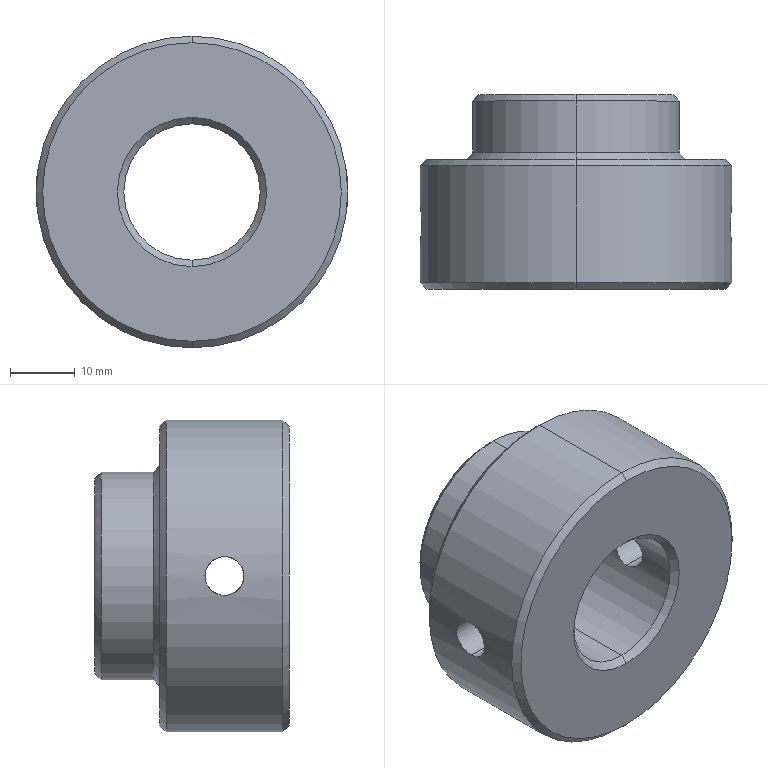Part | SolidWorks | features ICE 3, Chamfer 2, Extrusion 1 | 1 solid | 25 faces | box 48 x 30 x 48 mm | volume 32861 mm3 | cone 12 | cylinder 10 | plane 3 | commonest cylinder face diameters 6 x4 21 x2 32 x2 48 x2
STEP:
#1=CARTESIAN_POINT('',(0.,29.,-10.5));
#2=VERTEX_POINT('',#1);
#3=CARTESIAN_POINT('',(0.,29.,10.5));
#4=VERTEX_POINT('',#3);
#5=CARTESIAN_POINT('',(0.,29.,0.));
#6=DIRECTION('',(0.,1.,0.));
#7=DIRECTION('',(0.,0.,1.));
#8=AXIS2_PLACEMENT_3D('',#5,#6,#7);
#9=CIRCLE('',#8,10.5);
#10=EDGE_CURVE('',#2,#4,#9,.T.);
#11=ORIENTED_EDGE('',*,*,#10,.F.);
#12=CARTESIAN_POINT('',(0.,30.,-11.5));
#13=VERTEX_POINT('',#12);
#14=CARTESIAN_POINT('',(0.,29.,-10.5));
#15=DIRECTION('',(0.,0.7071,-0.7071));
#16=VECTOR('',#15,1000.);
#17=LINE('',#14,#16);
#18=EDGE_CURVE('',#2,#13,#17,.T.);
#19=ORIENTED_EDGE('',*,*,#18,.T.);
#20=CARTESIAN_POINT('',(0.,30.,11.5));
#21=VERTEX_POINT('',#20);
#22=CARTESIAN_POINT('',(0.,30.,0.));
#23=DIRECTION('',(0.,-1.,0.));
#24=DIRECTION('',(0.,0.,1.));
#25=AXIS2_PLACEMENT_3D('',#22,#23,#24);
#26=CIRCLE('',#25,11.5);
#27=EDGE_CURVE('',#21,#13,#26,.T.);
#28=ORIENTED_EDGE('',*,*,#27,.F.);
#29=CARTESIAN_POINT('',(0.,29.,10.5));
#30=DIRECTION('',(0.,0.7071,0.7071));
#31=VECTOR('',#30,1000.);
#32=LINE('',#29,#31);
#33=EDGE_CURVE('',#4,#21,#32,.T.);
#34=ORIENTED_EDGE('',*,*,#33,.F.);
#35=EDGE_LOOP('',(#11,#19,#28,#34));
#36=FACE_OUTER_BOUND('',#35,.T.);
#37=CARTESIAN_POINT('',(0.,29.,0.));
#38=DIRECTION('',(0.,1.,0.));
#39=DIRECTION('',(0.,0.,1.));
#40=AXIS2_PLACEMENT_3D('',#37,#38,#39);
#41=CONICAL_SURFACE('',#40,10.5,0.7854);
#42=ADVANCED_FACE('',(#36),#41,.F.);
#43=CARTESIAN_POINT('',(0.,0.,-23.));
#44=VERTEX_POINT('',#43);
#45=CARTESIAN_POINT('',(0.,0.,23.));
#46=VERTEX_POINT('',#45);
#47=CARTESIAN_POINT('',(0.,0.,0.));
#48=DIRECTION('',(0.,-1.,0.));
#49=DIRECTION('',(0.,0.,1.));
#50=AXIS2_PLACEMENT_3D('',#47,#48,#49);
#51=CIRCLE('',#50,23.);
#52=EDGE_CURVE('',#44,#46,#51,.T.);
#53=ORIENTED_EDGE('',*,*,#52,.F.);
#54=CARTESIAN_POINT('',(0.,1.,-24.));
#55=VERTEX_POINT('',#54);
#56=CARTESIAN_POINT('',(0.,1.,-24.));
#57=DIRECTION('',(0.,0.7071,-0.7071));
#58=VECTOR('',#57,1000.);
#59=LINE('',#56,#58);
#60=EDGE_CURVE('',#44,#55,#59,.T.);
#61=ORIENTED_EDGE('',*,*,#60,.T.);
#62=CARTESIAN_POINT('',(0.,1.,24.));
#63=VERTEX_POINT('',#62);
#64=CARTESIAN_POINT('',(0.,1.,0.));
#65=DIRECTION('',(0.,1.,0.));
#66=DIRECTION('',(0.,0.,1.));
#67=AXIS2_PLACEMENT_3D('',#64,#65,#66);
#68=CIRCLE('',#67,24.);
#69=EDGE_CURVE('',#63,#55,#68,.T.);
#70=ORIENTED_EDGE('',*,*,#69,.F.);
#71=CARTESIAN_POINT('',(0.,1.,24.));
#72=DIRECTION('',(0.,0.7071,0.7071));
#73=VECTOR('',#72,1000.);
#74=LINE('',#71,#73);
#75=EDGE_CURVE('',#46,#63,#74,.T.);
#76=ORIENTED_EDGE('',*,*,#75,.F.);
#77=EDGE_LOOP('',(#53,#61,#70,#76));
#78=FACE_OUTER_BOUND('',#77,.T.);
#79=CARTESIAN_POINT('',(0.,1.,0.));
#80=DIRECTION('',(0.,1.,0.));
#81=DIRECTION('',(0.,0.,1.));
#82=AXIS2_PLACEMENT_3D('',#79,#80,#81);
#83=CONICAL_SURFACE('',#82,24.,0.7854);
#84=ADVANCED_FACE('',(#78),#83,.T.);
#85=CARTESIAN_POINT('',(0.,20.,23.));
#86=VERTEX_POINT('',#85);
#87=CARTESIAN_POINT('',(0.,20.,-23.));
#88=VERTEX_POINT('',#87);
#89=CARTESIAN_POINT('',(0.,20.,0.));
#90=DIRECTION('',(0.,1.,0.));
#91=DIRECTION('',(0.,0.,1.));
#92=AXIS2_PLACEMENT_3D('',#89,#90,#91);
#93=CIRCLE('',#92,23.);
#94=EDGE_CURVE('',#86,#88,#93,.T.);
#95=ORIENTED_EDGE('',*,*,#94,.F.);
#96=CARTESIAN_POINT('',(0.,19.,24.));
#97=VERTEX_POINT('',#96);
#98=CARTESIAN_POINT('',(0.,20.,23.));
#99=DIRECTION('',(0.,-0.7071,0.7071));
#100=VECTOR('',#99,1000.);
#101=LINE('',#98,#100);
#102=EDGE_CURVE('',#86,#97,#101,.T.);
#103=ORIENTED_EDGE('',*,*,#102,.T.);
#104=CARTESIAN_POINT('',(0.,19.,-24.));
#105=VERTEX_POINT('',#104);
#106=CARTESIAN_POINT('',(0.,19.,0.));
#107=DIRECTION('',(0.,-1.,0.));
#108=DIRECTION('',(0.,0.,1.));
#109=AXIS2_PLACEMENT_3D('',#106,#107,#108);
#110=CIRCLE('',#109,24.);
#111=EDGE_CURVE('',#105,#97,#110,.T.);
#112=ORIENTED_EDGE('',*,*,#111,.F.);
#113=CARTESIAN_POINT('',(0.,20.,-23.));
#114=DIRECTION('',(0.,-0.7071,-0.7071));
#115=VECTOR('',#114,1000.);
#116=LINE('',#113,#115);
#117=EDGE_CURVE('',#88,#105,#116,.T.);
#118=ORIENTED_EDGE('',*,*,#117,.F.);
#119=EDGE_LOOP('',(#95,#103,#112,#118));
#120=FACE_OUTER_BOUND('',#119,.T.);
#121=CARTESIAN_POINT('',(0.,20.,0.));
#122=DIRECTION('',(0.,-1.,0.));
#123=DIRECTION('',(0.,0.,-1.));
#124=AXIS2_PLACEMENT_3D('',#121,#122,#123);
#125=CONICAL_SURFACE('',#124,23.,0.7854);
#126=ADVANCED_FACE('',(#120),#125,.T.);
#127=CARTESIAN_POINT('',(0.,30.,15.));
#128=VERTEX_POINT('',#127);
#129=CARTESIAN_POINT('',(0.,30.,-15.));
#130=VERTEX_POINT('',#129);
#131=CARTESIAN_POINT('',(0.,30.,0.));
#132=DIRECTION('',(0.,1.,0.));
#133=DIRECTION('',(0.,0.,1.));
#134=AXIS2_PLACEMENT_3D('',#131,#132,#133);
#135=CIRCLE('',#134,15.);
#136=EDGE_CURVE('',#128,#130,#135,.T.);
#137=ORIENTED_EDGE('',*,*,#136,.F.);
#138=CARTESIAN_POINT('',(0.,29.,16.));
#139=VERTEX_POINT('',#138);
#140=CARTESIAN_POINT('',(0.,30.,15.));
#141=DIRECTION('',(0.,-0.7071,0.7071));
#142=VECTOR('',#141,1000.);
#143=LINE('',#140,#142);
#144=EDGE_CURVE('',#128,#139,#143,.T.);
#145=ORIENTED_EDGE('',*,*,#144,.T.);
#146=CARTESIAN_POINT('',(0.,29.,-16.));
#147=VERTEX_POINT('',#146);
#148=CARTESIAN_POINT('',(0.,29.,0.));
#149=DIRECTION('',(0.,-1.,0.));
#150=DIRECTION('',(0.,0.,1.));
#151=AXIS2_PLACEMENT_3D('',#148,#149,#150);
#152=CIRCLE('',#151,16.);
#153=EDGE_CURVE('',#147,#139,#152,.T.);
#154=ORIENTED_EDGE('',*,*,#153,.F.);
#155=CARTESIAN_POINT('',(0.,30.,-15.));
#156=DIRECTION('',(0.,-0.7071,-0.7071));
#157=VECTOR('',#156,1000.);
#158=LINE('',#155,#157);
#159=EDGE_CURVE('',#130,#147,#158,.T.);
#160=ORIENTED_EDGE('',*,*,#159,.F.);
#161=EDGE_LOOP('',(#137,#145,#154,#160));
#162=FACE_OUTER_BOUND('',#161,.T.);
#163=CARTESIAN_POINT('',(0.,30.,0.));
#164=DIRECTION('',(0.,-1.,0.));
#165=DIRECTION('',(0.,0.,-1.));
#166=AXIS2_PLACEMENT_3D('',#163,#164,#165);
#167=CONICAL_SURFACE('',#166,15.,0.7854);
#168=ADVANCED_FACE('',(#162),#167,.T.);
#169=CARTESIAN_POINT('',(0.,21.,16.));
#170=VERTEX_POINT('',#169);
#171=CARTESIAN_POINT('',(0.,21.,-16.));
#172=VERTEX_POINT('',#171);
#173=CARTESIAN_POINT('',(0.,21.,0.));
#174=DIRECTION('',(0.,1.,0.));
#175=DIRECTION('',(0.,0.,1.));
#176=AXIS2_PLACEMENT_3D('',#173,#174,#175);
#177=CIRCLE('',#176,16.);
#178=EDGE_CURVE('',#170,#172,#177,.T.);
#179=ORIENTED_EDGE('',*,*,#178,.F.);
#180=CARTESIAN_POINT('',(0.,20.,17.));
#181=VERTEX_POINT('',#180);
#182=CARTESIAN_POINT('',(0.,21.,16.));
#183=DIRECTION('',(0.,-0.7071,0.7071));
#184=VECTOR('',#183,1000.);
#185=LINE('',#182,#184);
#186=EDGE_CURVE('',#170,#181,#185,.T.);
#187=ORIENTED_EDGE('',*,*,#186,.T.);
#188=CARTESIAN_POINT('',(0.,20.,-17.));
#189=VERTEX_POINT('',#188);
#190=CARTESIAN_POINT('',(0.,20.,0.));
#191=DIRECTION('',(0.,-1.,0.));
#192=DIRECTION('',(0.,0.,1.));
#193=AXIS2_PLACEMENT_3D('',#190,#191,#192);
#194=CIRCLE('',#193,17.);
#195=EDGE_CURVE('',#189,#181,#194,.T.);
#196=ORIENTED_EDGE('',*,*,#195,.F.);
#197=CARTESIAN_POINT('',(0.,21.,-16.));
#198=DIRECTION('',(0.,-0.7071,-0.7071));
#199=VECTOR('',#198,1000.);
#200=LINE('',#197,#199);
#201=EDGE_CURVE('',#172,#189,#200,.T.);
#202=ORIENTED_EDGE('',*,*,#201,.F.);
#203=EDGE_LOOP('',(#179,#187,#196,#202));
#204=FACE_OUTER_BOUND('',#203,.T.);
#205=CARTESIAN_POINT('',(0.,21.,0.));
#206=DIRECTION('',(0.,-1.,0.));
#207=DIRECTION('',(0.,0.,-1.));
#208=AXIS2_PLACEMENT_3D('',#205,#206,#207);
#209=CONICAL_SURFACE('',#208,16.,0.7854);
#210=ADVANCED_FACE('',(#204),#209,.T.);
#211=CARTESIAN_POINT('',(0.,1.,10.5));
#212=VERTEX_POINT('',#211);
#213=CARTESIAN_POINT('',(0.,1.,-10.5));
#214=VERTEX_POINT('',#213);
#215=CARTESIAN_POINT('',(0.,1.,0.));
#216=DIRECTION('',(0.,-1.,0.));
#217=DIRECTION('',(0.,0.,1.));
#218=AXIS2_PLACEMENT_3D('',#215,#216,#217);
#219=CIRCLE('',#218,10.5);
#220=EDGE_CURVE('',#212,#214,#219,.T.);
#221=ORIENTED_EDGE('',*,*,#220,.F.);
#222=CARTESIAN_POINT('',(0.,0.,11.5));
#223=VERTEX_POINT('',#222);
#224=CARTESIAN_POINT('',(0.,0.,11.5));
#225=DIRECTION('',(0.,-0.7071,0.7071));
#226=VECTOR('',#225,1000.);
#227=LINE('',#224,#226);
#228=EDGE_CURVE('',#212,#223,#227,.T.);
#229=ORIENTED_EDGE('',*,*,#228,.T.);
#230=CARTESIAN_POINT('',(0.,0.,-11.5));
#231=VERTEX_POINT('',#230);
#232=CARTESIAN_POINT('',(0.,0.,0.));
#233=DIRECTION('',(0.,1.,0.));
#234=DIRECTION('',(0.,0.,1.));
#235=AXIS2_PLACEMENT_3D('',#232,#233,#234);
#236=CIRCLE('',#235,11.5);
#237=EDGE_CURVE('',#231,#223,#236,.T.);
#238=ORIENTED_EDGE('',*,*,#237,.F.);
#239=CARTESIAN_POINT('',(0.,0.,-11.5));
#240=DIRECTION('',(0.,-0.7071,-0.7071));
#241=VECTOR('',#240,1000.);
#242=LINE('',#239,#241);
#243=EDGE_CURVE('',#214,#231,#242,.T.);
#244=ORIENTED_EDGE('',*,*,#243,.F.);
#245=EDGE_LOOP('',(#221,#229,#238,#244));
#246=FACE_OUTER_BOUND('',#245,.T.);
#247=CARTESIAN_POINT('',(0.,0.,0.));
#248=DIRECTION('',(0.,-1.,0.));
#249=DIRECTION('',(0.,0.,-1.));
#250=AXIS2_PLACEMENT_3D('',#247,#248,#249);
#251=CONICAL_SURFACE('',#250,11.5,0.7854);
#252=ADVANCED_FACE('',(#246),#251,.F.);
#253=CARTESIAN_POINT('',(-10.062,10.,3.));
#254=VERTEX_POINT('',#253);
#255=CARTESIAN_POINT('',(-10.062,10.,-3.));
#256=VERTEX_POINT('',#255);
#257=CARTESIAN_POINT('',(-10.062,10.,3.));
#258=CARTESIAN_POINT('',(-10.062,10.199,3.));
#259=CARTESIAN_POINT('',(-10.068,10.395,2.98));
#260=CARTESIAN_POINT('',(-10.091,10.78,2.903));
#261=CARTESIAN_POINT('',(-10.107,10.971,2.845));
#262=CARTESIAN_POINT('',(-10.149,11.334,2.694));
#263=CARTESIAN_POINT('',(-10.173,11.506,2.602));
#264=CARTESIAN_POINT('',(-10.226,11.831,2.384));
#265=CARTESIAN_POINT('',(-10.255,11.984,2.258));
#266=CARTESIAN_POINT('',(-10.34,12.397,1.846));
#267=CARTESIAN_POINT('',(-10.397,12.62,1.513));
#268=CARTESIAN_POINT('',(-10.457,12.845,0.9716));
#269=CARTESIAN_POINT('',(-10.473,12.903,0.7813));
#270=CARTESIAN_POINT('',(-10.494,12.981,0.3935));
#271=CARTESIAN_POINT('',(-10.5,13.,0.1981));
#272=CARTESIAN_POINT('',(-10.5,13.,-0.1956));
#273=CARTESIAN_POINT('',(-10.494,12.98,-0.3956));
#274=CARTESIAN_POINT('',(-10.473,12.903,-0.7812));
#275=CARTESIAN_POINT('',(-10.457,12.846,-0.9688));
#276=CARTESIAN_POINT('',(-10.396,12.619,-1.516));
#277=CARTESIAN_POINT('',(-10.34,12.398,-1.845));
#278=CARTESIAN_POINT('',(-10.255,11.982,-2.261));
#279=CARTESIAN_POINT('',(-10.226,11.831,-2.384));
#280=CARTESIAN_POINT('',(-10.173,11.507,-2.601));
#281=CARTESIAN_POINT('',(-10.148,11.331,-2.695));
#282=CARTESIAN_POINT('',(-10.107,10.97,-2.846));
#283=CARTESIAN_POINT('',(-10.091,10.783,-2.903));
#284=CARTESIAN_POINT('',(-10.068,10.396,-2.98));
#285=CARTESIAN_POINT('',(-10.062,10.196,-3.));
#286=CARTESIAN_POINT('',(-10.062,10.,-3.));
#287=B_SPLINE_CURVE_WITH_KNOTS('',3,(#257,#258,#259,#260,#261,#262,#263,#264,#265,#266,#267,#268,#269,#270,#271,#272,#273,#274,#275,#276,#277,#278,#279,#280,#281,#282,#283,#284,#285,#286),.UNSPECIFIED.,.F.,.F.,(4,2,2,2,2,2,2,2,2,2,2,2,2,2,4),(0.,0.0005893,0.001179,0.001768,0.002357,0.003536,0.004125,0.004714,0.005304,0.005893,0.007071,0.007661,0.00825,0.008839,0.009429),.UNSPECIFIED.);
#288=EDGE_CURVE('',#254,#256,#287,.T.);
#289=ORIENTED_EDGE('',*,*,#288,.T.);
#290=CARTESIAN_POINT('',(-10.062,10.,-3.));
#291=CARTESIAN_POINT('',(-10.062,9.804,-3.));
#292=CARTESIAN_POINT('',(-10.068,9.607,-2.981));
#293=CARTESIAN_POINT('',(-10.091,9.217,-2.903));
#294=CARTESIAN_POINT('',(-10.107,9.03,-2.846));
#295=CARTESIAN_POINT('',(-10.148,8.668,-2.695));
#296=CARTESIAN_POINT('',(-10.173,8.493,-2.601));
#297=CARTESIAN_POINT('',(-10.226,8.168,-2.384));
#298=CARTESIAN_POINT('',(-10.255,8.018,-2.26));
#299=CARTESIAN_POINT('',(-10.312,7.741,-1.984));
#300=CARTESIAN_POINT('',(-10.34,7.615,-1.831));
#301=CARTESIAN_POINT('',(-10.393,7.399,-1.507));
#302=CARTESIAN_POINT('',(-10.416,7.306,-1.335));
#303=CARTESIAN_POINT('',(-10.457,7.154,-0.9693));
#304=CARTESIAN_POINT('',(-10.473,7.097,-0.7815));
#305=CARTESIAN_POINT('',(-10.494,7.02,-0.3971));
#306=CARTESIAN_POINT('',(-10.5,7.,-0.1981));
#307=CARTESIAN_POINT('',(-10.5,7.,0.1973));
#308=CARTESIAN_POINT('',(-10.494,7.019,0.3928));
#309=CARTESIAN_POINT('',(-10.473,7.096,0.779));
#310=CARTESIAN_POINT('',(-10.457,7.155,0.9704));
#311=CARTESIAN_POINT('',(-10.397,7.38,1.513));
#312=CARTESIAN_POINT('',(-10.34,7.603,1.846));
#313=CARTESIAN_POINT('',(-10.255,8.016,2.258));
#314=CARTESIAN_POINT('',(-10.226,8.168,2.384));
#315=CARTESIAN_POINT('',(-10.173,8.494,2.602));
#316=CARTESIAN_POINT('',(-10.149,8.666,2.694));
#317=CARTESIAN_POINT('',(-10.108,9.027,2.845));
#318=CARTESIAN_POINT('',(-10.091,9.219,2.903));
#319=CARTESIAN_POINT('',(-10.068,9.605,2.98));
#320=CARTESIAN_POINT('',(-10.062,9.801,3.));
#321=CARTESIAN_POINT('',(-10.062,10.,3.));
#322=B_SPLINE_CURVE_WITH_KNOTS('',3,(#290,#291,#292,#293,#294,#295,#296,#297,#298,#299,#300,#301,#302,#303,#304,#305,#306,#307,#308,#309,#310,#311,#312,#313,#314,#315,#316,#317,#318,#319,#320,#321),.UNSPECIFIED.,.F.,.F.,(4,2,2,2,2,2,2,2,2,2,2,2,2,2,2,4),(0.009429,0.01002,0.01061,0.0112,0.01179,0.01237,0.01296,0.01355,0.01414,0.01473,0.01532,0.0165,0.01709,0.01768,0.01827,0.01885),.UNSPECIFIED.);
#323=EDGE_CURVE('',#256,#254,#322,.T.);
#324=ORIENTED_EDGE('',*,*,#323,.T.);
#325=EDGE_LOOP('',(#289,#324));
#326=FACE_BOUND('',#325,.T.);
#327=ORIENTED_EDGE('',*,*,#220,.T.);
#328=CARTESIAN_POINT('',(0.,0.,-10.5));
#329=DIRECTION('',(0.,1.,0.));
#330=VECTOR('',#329,1000.);
#331=LINE('',#328,#330);
#332=EDGE_CURVE('',#214,#2,#331,.T.);
#333=ORIENTED_EDGE('',*,*,#332,.T.);
#334=ORIENTED_EDGE('',*,*,#10,.T.);
#335=CARTESIAN_POINT('',(0.,0.,10.5));
#336=DIRECTION('',(0.,1.,0.));
#337=VECTOR('',#336,1000.);
#338=LINE('',#335,#337);
#339=EDGE_CURVE('',#212,#4,#338,.T.);
#340=ORIENTED_EDGE('',*,*,#339,.F.);
#341=EDGE_LOOP('',(#327,#333,#334,#340));
#342=FACE_OUTER_BOUND('',#341,.T.);
#343=CARTESIAN_POINT('',(0.,0.,0.));
#344=DIRECTION('',(0.,1.,0.));
#345=DIRECTION('',(0.,0.,1.));
#346=AXIS2_PLACEMENT_3D('',#343,#344,#345);
#347=CYLINDRICAL_SURFACE('',#346,10.5);
#348=ADVANCED_FACE('',(#326,#342),#347,.F.);
#349=ORIENTED_EDGE('',*,*,#153,.T.);
#350=CARTESIAN_POINT('',(0.,30.,16.));
#351=DIRECTION('',(0.,-1.,0.));
#352=VECTOR('',#351,1000.);
#353=LINE('',#350,#352);
#354=EDGE_CURVE('',#139,#170,#353,.T.);
#355=ORIENTED_EDGE('',*,*,#354,.T.);
#356=ORIENTED_EDGE('',*,*,#178,.T.);
#357=CARTESIAN_POINT('',(0.,30.,-16.));
#358=DIRECTION('',(0.,-1.,0.));
#359=VECTOR('',#358,1000.);
#360=LINE('',#357,#359);
#361=EDGE_CURVE('',#147,#172,#360,.T.);
#362=ORIENTED_EDGE('',*,*,#361,.F.);
#363=EDGE_LOOP('',(#349,#355,#356,#362));
#364=FACE_OUTER_BOUND('',#363,.T.);
#365=CARTESIAN_POINT('',(0.,30.,0.));
#366=DIRECTION('',(0.,-1.,0.));
#367=DIRECTION('',(0.,0.,-1.));
#368=AXIS2_PLACEMENT_3D('',#365,#366,#367);
#369=CYLINDRICAL_SURFACE('',#368,16.);
#370=ADVANCED_FACE('',(#364),#369,.T.);
#371=ORIENTED_EDGE('',*,*,#323,.F.);
#372=CARTESIAN_POINT('',(-23.812,10.,-3.));
#373=VERTEX_POINT('',#372);
#374=CARTESIAN_POINT('',(30.,10.,-3.));
#375=DIRECTION('',(-1.,0.,0.));
#376=VECTOR('',#375,1000.);
#377=LINE('',#374,#376);
#378=EDGE_CURVE('',#256,#373,#377,.T.);
#379=ORIENTED_EDGE('',*,*,#378,.T.);
#380=CARTESIAN_POINT('',(-23.812,10.,3.));
#381=VERTEX_POINT('',#380);
#382=CARTESIAN_POINT('',(-23.812,10.,-3.));
#383=CARTESIAN_POINT('',(-23.812,9.804,-3.));
#384=CARTESIAN_POINT('',(-23.814,9.609,-2.981));
#385=CARTESIAN_POINT('',(-23.824,9.222,-2.904));
#386=CARTESIAN_POINT('',(-23.831,9.033,-2.847));
#387=CARTESIAN_POINT('',(-23.848,8.672,-2.697));
#388=CARTESIAN_POINT('',(-23.859,8.497,-2.604));
#389=CARTESIAN_POINT('',(-23.881,8.169,-2.385));
#390=CARTESIAN_POINT('',(-23.894,8.018,-2.261));
#391=CARTESIAN_POINT('',(-23.918,7.742,-1.985));
#392=CARTESIAN_POINT('',(-23.931,7.615,-1.83));
#393=CARTESIAN_POINT('',(-23.953,7.397,-1.505));
#394=CARTESIAN_POINT('',(-23.964,7.305,-1.333));
#395=CARTESIAN_POINT('',(-23.981,7.154,-0.9695));
#396=CARTESIAN_POINT('',(-23.988,7.096,-0.7791));
#397=CARTESIAN_POINT('',(-23.998,7.02,-0.3956));
#398=CARTESIAN_POINT('',(-24.,7.,-0.2005));
#399=CARTESIAN_POINT('',(-24.,7.,0.1962));
#400=CARTESIAN_POINT('',(-23.998,7.019,0.3912));
#401=CARTESIAN_POINT('',(-23.988,7.095,0.775));
#402=CARTESIAN_POINT('',(-23.981,7.153,0.9657));
#403=CARTESIAN_POINT('',(-23.964,7.303,1.329));
#404=CARTESIAN_POINT('',(-23.954,7.395,1.501));
#405=CARTESIAN_POINT('',(-23.931,7.613,1.827));
#406=CARTESIAN_POINT('',(-23.918,7.739,1.982));
#407=CARTESIAN_POINT('',(-23.894,8.015,2.258));
#408=CARTESIAN_POINT('',(-23.882,8.166,2.382));
#409=CARTESIAN_POINT('',(-23.859,8.494,2.602));
#410=CARTESIAN_POINT('',(-23.848,8.668,2.695));
#411=CARTESIAN_POINT('',(-23.831,9.029,2.845));
#412=CARTESIAN_POINT('',(-23.824,9.218,2.903));
#413=CARTESIAN_POINT('',(-23.814,9.606,2.981));
#414=CARTESIAN_POINT('',(-23.812,9.802,3.));
#415=CARTESIAN_POINT('',(-23.812,10.,3.));
#416=B_SPLINE_CURVE_WITH_KNOTS('',3,(#382,#383,#384,#385,#386,#387,#388,#389,#390,#391,#392,#393,#394,#395,#396,#397,#398,#399,#400,#401,#402,#403,#404,#405,#406,#407,#408,#409,#410,#411,#412,#413,#414,#415),.UNSPECIFIED.,.F.,.F.,(4,2,2,2,2,2,2,2,2,2,2,2,2,2,2,2,4),(0.009389,0.009975,0.01056,0.01115,0.01174,0.01232,0.01291,0.0135,0.01408,0.01467,0.01525,0.01584,0.01643,0.01701,0.0176,0.01819,0.01877),.UNSPECIFIED.);
#417=EDGE_CURVE('',#373,#381,#416,.T.);
#418=ORIENTED_EDGE('',*,*,#417,.T.);
#419=CARTESIAN_POINT('',(30.,10.,3.));
#420=DIRECTION('',(-1.,0.,0.));
#421=VECTOR('',#420,1000.);
#422=LINE('',#419,#421);
#423=EDGE_CURVE('',#254,#381,#422,.T.);
#424=ORIENTED_EDGE('',*,*,#423,.F.);
#425=EDGE_LOOP('',(#371,#379,#418,#424));
#426=FACE_OUTER_BOUND('',#425,.T.);
#427=CARTESIAN_POINT('',(30.,10.,0.));
#428=DIRECTION('',(-1.,0.,0.));
#429=DIRECTION('',(0.,0.,1.));
#430=AXIS2_PLACEMENT_3D('',#427,#428,#429);
#431=CYLINDRICAL_SURFACE('',#430,3.);
#432=ADVANCED_FACE('',(#426),#431,.F.);
#433=CARTESIAN_POINT('',(23.812,10.,3.));
#434=VERTEX_POINT('',#433);
#435=CARTESIAN_POINT('',(23.812,10.,-3.));
#436=VERTEX_POINT('',#435);
#437=CARTESIAN_POINT('',(23.812,10.,3.));
#438=CARTESIAN_POINT('',(23.812,9.802,3.));
#439=CARTESIAN_POINT('',(23.814,9.607,2.981));
#440=CARTESIAN_POINT('',(23.824,9.223,2.904));
#441=CARTESIAN_POINT('',(23.831,9.032,2.846));
#442=CARTESIAN_POINT('',(23.848,8.669,2.696));
#443=CARTESIAN_POINT('',(23.859,8.497,2.604));
#444=CARTESIAN_POINT('',(23.881,8.171,2.386));
#445=CARTESIAN_POINT('',(23.894,8.016,2.259));
#446=CARTESIAN_POINT('',(23.918,7.74,1.983));
#447=CARTESIAN_POINT('',(23.931,7.616,1.832));
#448=CARTESIAN_POINT('',(23.953,7.397,1.504));
#449=CARTESIAN_POINT('',(23.964,7.304,1.329));
#450=CARTESIAN_POINT('',(23.981,7.154,0.9685));
#451=CARTESIAN_POINT('',(23.988,7.096,0.7792));
#452=CARTESIAN_POINT('',(23.998,7.019,0.3918));
#453=CARTESIAN_POINT('',(24.,7.,0.197));
#454=CARTESIAN_POINT('',(24.,7.,-0.1948));
#455=CARTESIAN_POINT('',(23.998,7.019,-0.3938));
#456=CARTESIAN_POINT('',(23.988,7.096,-0.7787));
#457=CARTESIAN_POINT('',(23.981,7.153,-0.9658));
#458=CARTESIAN_POINT('',(23.964,7.303,-1.329));
#459=CARTESIAN_POINT('',(23.953,7.397,-1.505));
#460=CARTESIAN_POINT('',(23.931,7.614,-1.83));
#461=CARTESIAN_POINT('',(23.919,7.739,-1.981));
#462=CARTESIAN_POINT('',(23.894,8.018,-2.261));
#463=CARTESIAN_POINT('',(23.881,8.17,-2.385));
#464=CARTESIAN_POINT('',(23.859,8.495,-2.602));
#465=CARTESIAN_POINT('',(23.848,8.67,-2.696));
#466=CARTESIAN_POINT('',(23.831,9.033,-2.847));
#467=CARTESIAN_POINT('',(23.824,9.22,-2.904));
#468=CARTESIAN_POINT('',(23.814,9.605,-2.98));
#469=CARTESIAN_POINT('',(23.812,9.804,-3.));
#470=CARTESIAN_POINT('',(23.812,10.,-3.));
#471=B_SPLINE_CURVE_WITH_KNOTS('',3,(#437,#438,#439,#440,#441,#442,#443,#444,#445,#446,#447,#448,#449,#450,#451,#452,#453,#454,#455,#456,#457,#458,#459,#460,#461,#462,#463,#464,#465,#466,#467,#468,#469,#470),.UNSPECIFIED.,.F.,.F.,(4,2,2,2,2,2,2,2,2,2,2,2,2,2,2,2,4),(0.,0.0005868,0.001174,0.00176,0.002347,0.002934,0.003521,0.004107,0.004694,0.005281,0.005868,0.006455,0.007041,0.007628,0.008215,0.008802,0.009389),.UNSPECIFIED.);
#472=EDGE_CURVE('',#434,#436,#471,.T.);
#473=ORIENTED_EDGE('',*,*,#472,.F.);
#474=CARTESIAN_POINT('',(23.812,10.,-3.));
#475=CARTESIAN_POINT('',(23.812,10.196,-3.));
#476=CARTESIAN_POINT('',(23.814,10.391,-2.981));
#477=CARTESIAN_POINT('',(23.824,10.778,-2.904));
#478=CARTESIAN_POINT('',(23.831,10.967,-2.847));
#479=CARTESIAN_POINT('',(23.848,11.328,-2.697));
#480=CARTESIAN_POINT('',(23.859,11.503,-2.604));
#481=CARTESIAN_POINT('',(23.881,11.831,-2.385));
#482=CARTESIAN_POINT('',(23.894,11.982,-2.261));
#483=CARTESIAN_POINT('',(23.918,12.258,-1.985));
#484=CARTESIAN_POINT('',(23.931,12.385,-1.83));
#485=CARTESIAN_POINT('',(23.953,12.603,-1.505));
#486=CARTESIAN_POINT('',(23.964,12.695,-1.333));
#487=CARTESIAN_POINT('',(23.981,12.846,-0.9695));
#488=CARTESIAN_POINT('',(23.988,12.904,-0.7791));
#489=CARTESIAN_POINT('',(23.998,12.98,-0.3956));
#490=CARTESIAN_POINT('',(24.,13.,-0.2005));
#491=CARTESIAN_POINT('',(24.,13.,0.1962));
#492=CARTESIAN_POINT('',(23.998,12.981,0.3912));
#493=CARTESIAN_POINT('',(23.988,12.905,0.775));
#494=CARTESIAN_POINT('',(23.981,12.847,0.9657));
#495=CARTESIAN_POINT('',(23.964,12.697,1.329));
#496=CARTESIAN_POINT('',(23.954,12.605,1.501));
#497=CARTESIAN_POINT('',(23.931,12.387,1.827));
#498=CARTESIAN_POINT('',(23.918,12.261,1.982));
#499=CARTESIAN_POINT('',(23.894,11.985,2.258));
#500=CARTESIAN_POINT('',(23.882,11.834,2.382));
#501=CARTESIAN_POINT('',(23.859,11.506,2.602));
#502=CARTESIAN_POINT('',(23.848,11.332,2.695));
#503=CARTESIAN_POINT('',(23.831,10.971,2.845));
#504=CARTESIAN_POINT('',(23.824,10.782,2.903));
#505=CARTESIAN_POINT('',(23.814,10.394,2.981));
#506=CARTESIAN_POINT('',(23.812,10.198,3.));
#507=CARTESIAN_POINT('',(23.812,10.,3.));
#508=B_SPLINE_CURVE_WITH_KNOTS('',3,(#474,#475,#476,#477,#478,#479,#480,#481,#482,#483,#484,#485,#486,#487,#488,#489,#490,#491,#492,#493,#494,#495,#496,#497,#498,#499,#500,#501,#502,#503,#504,#505,#506,#507),.UNSPECIFIED.,.F.,.F.,(4,2,2,2,2,2,2,2,2,2,2,2,2,2,2,2,4),(0.009389,0.009975,0.01056,0.01115,0.01174,0.01232,0.01291,0.0135,0.01408,0.01467,0.01525,0.01584,0.01643,0.01701,0.0176,0.01819,0.01877),.UNSPECIFIED.);
#509=EDGE_CURVE('',#436,#434,#508,.T.);
#510=ORIENTED_EDGE('',*,*,#509,.F.);
#511=EDGE_LOOP('',(#473,#510));
#512=FACE_BOUND('',#511,.T.);
#513=ORIENTED_EDGE('',*,*,#111,.T.);
#514=CARTESIAN_POINT('',(0.,20.,24.));
#515=DIRECTION('',(0.,-1.,0.));
#516=VECTOR('',#515,1000.);
#517=LINE('',#514,#516);
#518=EDGE_CURVE('',#97,#63,#517,.T.);
#519=ORIENTED_EDGE('',*,*,#518,.T.);
#520=ORIENTED_EDGE('',*,*,#69,.T.);
#521=CARTESIAN_POINT('',(0.,20.,-24.));
#522=DIRECTION('',(0.,-1.,0.));
#523=VECTOR('',#522,1000.);
#524=LINE('',#521,#523);
#525=EDGE_CURVE('',#105,#55,#524,.T.);
#526=ORIENTED_EDGE('',*,*,#525,.F.);
#527=EDGE_LOOP('',(#513,#519,#520,#526));
#528=FACE_OUTER_BOUND('',#527,.T.);
#529=CARTESIAN_POINT('',(0.,20.,0.));
#530=DIRECTION('',(0.,-1.,0.));
#531=DIRECTION('',(0.,0.,-1.));
#532=AXIS2_PLACEMENT_3D('',#529,#530,#531);
#533=CYLINDRICAL_SURFACE('',#532,24.);
#534=ADVANCED_FACE('',(#512,#528),#533,.T.);
#535=ORIENTED_EDGE('',*,*,#472,.T.);
#536=CARTESIAN_POINT('',(10.062,10.,-3.));
#537=VERTEX_POINT('',#536);
#538=CARTESIAN_POINT('',(30.,10.,-3.));
#539=DIRECTION('',(-1.,0.,0.));
#540=VECTOR('',#539,1000.);
#541=LINE('',#538,#540);
#542=EDGE_CURVE('',#436,#537,#541,.T.);
#543=ORIENTED_EDGE('',*,*,#542,.T.);
#544=CARTESIAN_POINT('',(10.062,10.,3.));
#545=VERTEX_POINT('',#544);
#546=CARTESIAN_POINT('',(10.062,10.,3.));
#547=CARTESIAN_POINT('',(10.062,9.801,3.));
#548=CARTESIAN_POINT('',(10.068,9.605,2.98));
#549=CARTESIAN_POINT('',(10.091,9.22,2.903));
#550=CARTESIAN_POINT('',(10.107,9.029,2.845));
#551=CARTESIAN_POINT('',(10.149,8.666,2.694));
#552=CARTESIAN_POINT('',(10.173,8.494,2.602));
#553=CARTESIAN_POINT('',(10.226,8.169,2.384));
#554=CARTESIAN_POINT('',(10.255,8.016,2.258));
#555=CARTESIAN_POINT('',(10.34,7.603,1.846));
#556=CARTESIAN_POINT('',(10.397,7.38,1.513));
#557=CARTESIAN_POINT('',(10.457,7.155,0.9716));
#558=CARTESIAN_POINT('',(10.473,7.097,0.7813));
#559=CARTESIAN_POINT('',(10.494,7.019,0.3935));
#560=CARTESIAN_POINT('',(10.5,7.,0.1981));
#561=CARTESIAN_POINT('',(10.5,7.,-0.1956));
#562=CARTESIAN_POINT('',(10.494,7.02,-0.3956));
#563=CARTESIAN_POINT('',(10.473,7.097,-0.7812));
#564=CARTESIAN_POINT('',(10.457,7.154,-0.9688));
#565=CARTESIAN_POINT('',(10.396,7.381,-1.516));
#566=CARTESIAN_POINT('',(10.34,7.602,-1.845));
#567=CARTESIAN_POINT('',(10.255,8.018,-2.261));
#568=CARTESIAN_POINT('',(10.226,8.169,-2.384));
#569=CARTESIAN_POINT('',(10.173,8.493,-2.601));
#570=CARTESIAN_POINT('',(10.148,8.669,-2.695));
#571=CARTESIAN_POINT('',(10.107,9.03,-2.846));
#572=CARTESIAN_POINT('',(10.091,9.217,-2.903));
#573=CARTESIAN_POINT('',(10.068,9.604,-2.98));
#574=CARTESIAN_POINT('',(10.062,9.804,-3.));
#575=CARTESIAN_POINT('',(10.062,10.,-3.));
#576=B_SPLINE_CURVE_WITH_KNOTS('',3,(#546,#547,#548,#549,#550,#551,#552,#553,#554,#555,#556,#557,#558,#559,#560,#561,#562,#563,#564,#565,#566,#567,#568,#569,#570,#571,#572,#573,#574,#575),.UNSPECIFIED.,.F.,.F.,(4,2,2,2,2,2,2,2,2,2,2,2,2,2,4),(0.,0.0005893,0.001179,0.001768,0.002357,0.003536,0.004125,0.004714,0.005304,0.005893,0.007071,0.007661,0.00825,0.008839,0.009429),.UNSPECIFIED.);
#577=EDGE_CURVE('',#545,#537,#576,.T.);
#578=ORIENTED_EDGE('',*,*,#577,.F.);
#579=CARTESIAN_POINT('',(30.,10.,3.));
#580=DIRECTION('',(-1.,0.,0.));
#581=VECTOR('',#580,1000.);
#582=LINE('',#579,#581);
#583=EDGE_CURVE('',#434,#545,#582,.T.);
#584=ORIENTED_EDGE('',*,*,#583,.F.);
#585=EDGE_LOOP('',(#535,#543,#578,#584));
#586=FACE_OUTER_BOUND('',#585,.T.);
#587=CARTESIAN_POINT('',(30.,10.,0.));
#588=DIRECTION('',(-1.,0.,0.));
#589=DIRECTION('',(0.,0.,1.));
#590=AXIS2_PLACEMENT_3D('',#587,#588,#589);
#591=CYLINDRICAL_SURFACE('',#590,3.);
#592=ADVANCED_FACE('',(#586),#591,.F.);
#593=ORIENTED_EDGE('',*,*,#542,.F.);
#594=ORIENTED_EDGE('',*,*,#509,.T.);
#595=ORIENTED_EDGE('',*,*,#583,.T.);
#596=CARTESIAN_POINT('',(10.062,10.,-3.));
#597=CARTESIAN_POINT('',(10.062,10.196,-3.));
#598=CARTESIAN_POINT('',(10.068,10.393,-2.981));
#599=CARTESIAN_POINT('',(10.091,10.783,-2.903));
#600=CARTESIAN_POINT('',(10.107,10.97,-2.846));
#601=CARTESIAN_POINT('',(10.148,11.332,-2.695));
#602=CARTESIAN_POINT('',(10.173,11.507,-2.601));
#603=CARTESIAN_POINT('',(10.226,11.832,-2.384));
#604=CARTESIAN_POINT('',(10.255,11.982,-2.26));
#605=CARTESIAN_POINT('',(10.312,12.259,-1.984));
#606=CARTESIAN_POINT('',(10.34,12.385,-1.831));
#607=CARTESIAN_POINT('',(10.393,12.601,-1.507));
#608=CARTESIAN_POINT('',(10.416,12.694,-1.335));
#609=CARTESIAN_POINT('',(10.457,12.846,-0.9693));
#610=CARTESIAN_POINT('',(10.473,12.903,-0.7815));
#611=CARTESIAN_POINT('',(10.494,12.98,-0.3971));
#612=CARTESIAN_POINT('',(10.5,13.,-0.1981));
#613=CARTESIAN_POINT('',(10.5,13.,0.1973));
#614=CARTESIAN_POINT('',(10.494,12.981,0.3928));
#615=CARTESIAN_POINT('',(10.473,12.904,0.779));
#616=CARTESIAN_POINT('',(10.457,12.845,0.9704));
#617=CARTESIAN_POINT('',(10.397,12.62,1.513));
#618=CARTESIAN_POINT('',(10.34,12.397,1.846));
#619=CARTESIAN_POINT('',(10.255,11.984,2.258));
#620=CARTESIAN_POINT('',(10.226,11.832,2.384));
#621=CARTESIAN_POINT('',(10.173,11.506,2.602));
#622=CARTESIAN_POINT('',(10.149,11.334,2.694));
#623=CARTESIAN_POINT('',(10.108,10.973,2.845));
#624=CARTESIAN_POINT('',(10.091,10.781,2.903));
#625=CARTESIAN_POINT('',(10.068,10.395,2.98));
#626=CARTESIAN_POINT('',(10.062,10.199,3.));
#627=CARTESIAN_POINT('',(10.062,10.,3.));
#628=B_SPLINE_CURVE_WITH_KNOTS('',3,(#596,#597,#598,#599,#600,#601,#602,#603,#604,#605,#606,#607,#608,#609,#610,#611,#612,#613,#614,#615,#616,#617,#618,#619,#620,#621,#622,#623,#624,#625,#626,#627),.UNSPECIFIED.,.F.,.F.,(4,2,2,2,2,2,2,2,2,2,2,2,2,2,2,4),(0.009429,0.01002,0.01061,0.0112,0.01179,0.01237,0.01296,0.01355,0.01414,0.01473,0.01532,0.0165,0.01709,0.01768,0.01827,0.01885),.UNSPECIFIED.);
#629=EDGE_CURVE('',#537,#545,#628,.T.);
#630=ORIENTED_EDGE('',*,*,#629,.F.);
#631=EDGE_LOOP('',(#593,#594,#595,#630));
#632=FACE_OUTER_BOUND('',#631,.T.);
#633=CARTESIAN_POINT('',(30.,10.,0.));
#634=DIRECTION('',(-1.,0.,0.));
#635=DIRECTION('',(0.,0.,1.));
#636=AXIS2_PLACEMENT_3D('',#633,#634,#635);
#637=CYLINDRICAL_SURFACE('',#636,3.);
#638=ADVANCED_FACE('',(#632),#637,.F.);
#639=ORIENTED_EDGE('',*,*,#518,.F.);
#640=CARTESIAN_POINT('',(0.,19.,0.));
#641=DIRECTION('',(0.,-1.,0.));
#642=DIRECTION('',(0.,0.,1.));
#643=AXIS2_PLACEMENT_3D('',#640,#641,#642);
#644=CIRCLE('',#643,24.);
#645=EDGE_CURVE('',#97,#105,#644,.T.);
#646=ORIENTED_EDGE('',*,*,#645,.T.);
#647=ORIENTED_EDGE('',*,*,#525,.T.);
#648=CARTESIAN_POINT('',(0.,1.,0.));
#649=DIRECTION('',(0.,1.,0.));
#650=DIRECTION('',(0.,0.,1.));
#651=AXIS2_PLACEMENT_3D('',#648,#649,#650);
#652=CIRCLE('',#651,24.);
#653=EDGE_CURVE('',#55,#63,#652,.T.);
#654=ORIENTED_EDGE('',*,*,#653,.T.);
#655=EDGE_LOOP('',(#639,#646,#647,#654));
#656=FACE_OUTER_BOUND('',#655,.T.);
#657=CARTESIAN_POINT('',(-23.812,10.,3.));
#658=CARTESIAN_POINT('',(-23.812,10.198,3.));
#659=CARTESIAN_POINT('',(-23.814,10.393,2.981));
#660=CARTESIAN_POINT('',(-23.824,10.777,2.904));
#661=CARTESIAN_POINT('',(-23.831,10.968,2.846));
#662=CARTESIAN_POINT('',(-23.848,11.331,2.696));
#663=CARTESIAN_POINT('',(-23.859,11.503,2.604));
#664=CARTESIAN_POINT('',(-23.881,11.829,2.386));
#665=CARTESIAN_POINT('',(-23.894,11.984,2.259));
#666=CARTESIAN_POINT('',(-23.918,12.26,1.983));
#667=CARTESIAN_POINT('',(-23.931,12.384,1.832));
#668=CARTESIAN_POINT('',(-23.953,12.603,1.504));
#669=CARTESIAN_POINT('',(-23.964,12.696,1.329));
#670=CARTESIAN_POINT('',(-23.981,12.846,0.9685));
#671=CARTESIAN_POINT('',(-23.988,12.904,0.7792));
#672=CARTESIAN_POINT('',(-23.998,12.981,0.3918));
#673=CARTESIAN_POINT('',(-24.,13.,0.197));
#674=CARTESIAN_POINT('',(-24.,13.,-0.1948));
#675=CARTESIAN_POINT('',(-23.998,12.981,-0.3938));
#676=CARTESIAN_POINT('',(-23.988,12.904,-0.7787));
#677=CARTESIAN_POINT('',(-23.981,12.847,-0.9658));
#678=CARTESIAN_POINT('',(-23.964,12.697,-1.329));
#679=CARTESIAN_POINT('',(-23.953,12.603,-1.505));
#680=CARTESIAN_POINT('',(-23.931,12.386,-1.83));
#681=CARTESIAN_POINT('',(-23.919,12.261,-1.981));
#682=CARTESIAN_POINT('',(-23.894,11.982,-2.261));
#683=CARTESIAN_POINT('',(-23.881,11.83,-2.385));
#684=CARTESIAN_POINT('',(-23.859,11.505,-2.602));
#685=CARTESIAN_POINT('',(-23.848,11.33,-2.696));
#686=CARTESIAN_POINT('',(-23.831,10.967,-2.847));
#687=CARTESIAN_POINT('',(-23.824,10.78,-2.904));
#688=CARTESIAN_POINT('',(-23.814,10.395,-2.98));
#689=CARTESIAN_POINT('',(-23.812,10.196,-3.));
#690=CARTESIAN_POINT('',(-23.812,10.,-3.));
#691=B_SPLINE_CURVE_WITH_KNOTS('',3,(#657,#658,#659,#660,#661,#662,#663,#664,#665,#666,#667,#668,#669,#670,#671,#672,#673,#674,#675,#676,#677,#678,#679,#680,#681,#682,#683,#684,#685,#686,#687,#688,#689,#690),.UNSPECIFIED.,.F.,.F.,(4,2,2,2,2,2,2,2,2,2,2,2,2,2,2,2,4),(0.,0.0005868,0.001174,0.00176,0.002347,0.002934,0.003521,0.004107,0.004694,0.005281,0.005868,0.006455,0.007041,0.007628,0.008215,0.008802,0.009389),.UNSPECIFIED.);
#692=EDGE_CURVE('',#381,#373,#691,.T.);
#693=ORIENTED_EDGE('',*,*,#692,.F.);
#694=ORIENTED_EDGE('',*,*,#417,.F.);
#695=EDGE_LOOP('',(#693,#694));
#696=FACE_BOUND('',#695,.T.);
#697=CARTESIAN_POINT('',(0.,20.,0.));
#698=DIRECTION('',(0.,-1.,0.));
#699=DIRECTION('',(0.,0.,-1.));
#700=AXIS2_PLACEMENT_3D('',#697,#698,#699);
#701=CYLINDRICAL_SURFACE('',#700,24.);
#702=ADVANCED_FACE('',(#656,#696),#701,.T.);
#703=ORIENTED_EDGE('',*,*,#195,.T.);
#704=CARTESIAN_POINT('',(0.,20.,0.));
#705=DIRECTION('',(0.,-1.,0.));
#706=DIRECTION('',(0.,0.,1.));
#707=AXIS2_PLACEMENT_3D('',#704,#705,#706);
#708=CIRCLE('',#707,17.);
#709=EDGE_CURVE('',#181,#189,#708,.T.);
#710=ORIENTED_EDGE('',*,*,#709,.T.);
#711=EDGE_LOOP('',(#703,#710));
#712=FACE_BOUND('',#711,.T.);
#713=CARTESIAN_POINT('',(0.,20.,0.));
#714=DIRECTION('',(0.,1.,0.));
#715=DIRECTION('',(0.,0.,1.));
#716=AXIS2_PLACEMENT_3D('',#713,#714,#715);
#717=CIRCLE('',#716,23.);
#718=EDGE_CURVE('',#88,#86,#717,.T.);
#719=ORIENTED_EDGE('',*,*,#718,.T.);
#720=ORIENTED_EDGE('',*,*,#94,.T.);
#721=EDGE_LOOP('',(#719,#720));
#722=FACE_OUTER_BOUND('',#721,.T.);
#723=CARTESIAN_POINT('',(0.,20.,0.));
#724=DIRECTION('',(0.,1.,0.));
#725=DIRECTION('',(0.,0.,1.));
#726=AXIS2_PLACEMENT_3D('',#723,#724,#725);
#727=PLANE('',#726);
#728=ADVANCED_FACE('',(#712,#722),#727,.T.);
#729=ORIENTED_EDGE('',*,*,#237,.T.);
#730=CARTESIAN_POINT('',(0.,0.,0.));
#731=DIRECTION('',(0.,1.,0.));
#732=DIRECTION('',(0.,0.,1.));
#733=AXIS2_PLACEMENT_3D('',#730,#731,#732);
#734=CIRCLE('',#733,11.5);
#735=EDGE_CURVE('',#223,#231,#734,.T.);
#736=ORIENTED_EDGE('',*,*,#735,.T.);
#737=EDGE_LOOP('',(#729,#736));
#738=FACE_BOUND('',#737,.T.);
#739=CARTESIAN_POINT('',(0.,0.,0.));
#740=DIRECTION('',(0.,-1.,0.));
#741=DIRECTION('',(0.,0.,1.));
#742=AXIS2_PLACEMENT_3D('',#739,#740,#741);
#743=CIRCLE('',#742,23.);
#744=EDGE_CURVE('',#46,#44,#743,.T.);
#745=ORIENTED_EDGE('',*,*,#744,.T.);
#746=ORIENTED_EDGE('',*,*,#52,.T.);
#747=EDGE_LOOP('',(#745,#746));
#748=FACE_OUTER_BOUND('',#747,.T.);
#749=CARTESIAN_POINT('',(0.,0.,0.));
#750=DIRECTION('',(0.,1.,0.));
#751=DIRECTION('',(0.,0.,1.));
#752=AXIS2_PLACEMENT_3D('',#749,#750,#751);
#753=PLANE('',#752);
#754=ADVANCED_FACE('',(#738,#748),#753,.F.);
#755=ORIENTED_EDGE('',*,*,#378,.F.);
#756=ORIENTED_EDGE('',*,*,#288,.F.);
#757=ORIENTED_EDGE('',*,*,#423,.T.);
#758=ORIENTED_EDGE('',*,*,#692,.T.);
#759=EDGE_LOOP('',(#755,#756,#757,#758));
#760=FACE_OUTER_BOUND('',#759,.T.);
#761=CARTESIAN_POINT('',(30.,10.,0.));
#762=DIRECTION('',(-1.,0.,0.));
#763=DIRECTION('',(0.,0.,1.));
#764=AXIS2_PLACEMENT_3D('',#761,#762,#763);
#765=CYLINDRICAL_SURFACE('',#764,3.);
#766=ADVANCED_FACE('',(#760),#765,.F.);
#767=ORIENTED_EDGE('',*,*,#354,.F.);
#768=CARTESIAN_POINT('',(0.,29.,0.));
#769=DIRECTION('',(0.,-1.,0.));
#770=DIRECTION('',(0.,0.,1.));
#771=AXIS2_PLACEMENT_3D('',#768,#769,#770);
#772=CIRCLE('',#771,16.);
#773=EDGE_CURVE('',#139,#147,#772,.T.);
#774=ORIENTED_EDGE('',*,*,#773,.T.);
#775=ORIENTED_EDGE('',*,*,#361,.T.);
#776=CARTESIAN_POINT('',(0.,21.,0.));
#777=DIRECTION('',(0.,1.,0.));
#778=DIRECTION('',(0.,0.,1.));
#779=AXIS2_PLACEMENT_3D('',#776,#777,#778);
#780=CIRCLE('',#779,16.);
#781=EDGE_CURVE('',#172,#170,#780,.T.);
#782=ORIENTED_EDGE('',*,*,#781,.T.);
#783=EDGE_LOOP('',(#767,#774,#775,#782));
#784=FACE_OUTER_BOUND('',#783,.T.);
#785=CARTESIAN_POINT('',(0.,30.,0.));
#786=DIRECTION('',(0.,-1.,0.));
#787=DIRECTION('',(0.,0.,-1.));
#788=AXIS2_PLACEMENT_3D('',#785,#786,#787);
#789=CYLINDRICAL_SURFACE('',#788,16.);
#790=ADVANCED_FACE('',(#784),#789,.T.);
#791=ORIENTED_EDGE('',*,*,#27,.T.);
#792=CARTESIAN_POINT('',(0.,30.,0.));
#793=DIRECTION('',(0.,-1.,0.));
#794=DIRECTION('',(0.,0.,1.));
#795=AXIS2_PLACEMENT_3D('',#792,#793,#794);
#796=CIRCLE('',#795,11.5);
#797=EDGE_CURVE('',#13,#21,#796,.T.);
#798=ORIENTED_EDGE('',*,*,#797,.T.);
#799=EDGE_LOOP('',(#791,#798));
#800=FACE_BOUND('',#799,.T.);
#801=CARTESIAN_POINT('',(0.,30.,0.));
#802=DIRECTION('',(0.,1.,0.));
#803=DIRECTION('',(0.,0.,1.));
#804=AXIS2_PLACEMENT_3D('',#801,#802,#803);
#805=CIRCLE('',#804,15.);
#806=EDGE_CURVE('',#130,#128,#805,.T.);
#807=ORIENTED_EDGE('',*,*,#806,.T.);
#808=ORIENTED_EDGE('',*,*,#136,.T.);
#809=EDGE_LOOP('',(#807,#808));
#810=FACE_OUTER_BOUND('',#809,.T.);
#811=CARTESIAN_POINT('',(0.,30.,0.));
#812=DIRECTION('',(0.,1.,0.));
#813=DIRECTION('',(0.,0.,1.));
#814=AXIS2_PLACEMENT_3D('',#811,#812,#813);
#815=PLANE('',#814);
#816=ADVANCED_FACE('',(#800,#810),#815,.T.);
#817=ORIENTED_EDGE('',*,*,#332,.F.);
#818=CARTESIAN_POINT('',(0.,1.,0.));
#819=DIRECTION('',(0.,-1.,0.));
#820=DIRECTION('',(0.,0.,1.));
#821=AXIS2_PLACEMENT_3D('',#818,#819,#820);
#822=CIRCLE('',#821,10.5);
#823=EDGE_CURVE('',#214,#212,#822,.T.);
#824=ORIENTED_EDGE('',*,*,#823,.T.);
#825=ORIENTED_EDGE('',*,*,#339,.T.);
#826=CARTESIAN_POINT('',(0.,29.,0.));
#827=DIRECTION('',(0.,1.,0.));
#828=DIRECTION('',(0.,0.,1.));
#829=AXIS2_PLACEMENT_3D('',#826,#827,#828);
#830=CIRCLE('',#829,10.5);
#831=EDGE_CURVE('',#4,#2,#830,.T.);
#832=ORIENTED_EDGE('',*,*,#831,.T.);
#833=EDGE_LOOP('',(#817,#824,#825,#832));
#834=FACE_OUTER_BOUND('',#833,.T.);
#835=ORIENTED_EDGE('',*,*,#577,.T.);
#836=ORIENTED_EDGE('',*,*,#629,.T.);
#837=EDGE_LOOP('',(#835,#836));
#838=FACE_BOUND('',#837,.T.);
#839=CARTESIAN_POINT('',(0.,0.,0.));
#840=DIRECTION('',(0.,1.,0.));
#841=DIRECTION('',(0.,0.,1.));
#842=AXIS2_PLACEMENT_3D('',#839,#840,#841);
#843=CYLINDRICAL_SURFACE('',#842,10.5);
#844=ADVANCED_FACE('',(#834,#838),#843,.F.);
#845=ORIENTED_EDGE('',*,*,#228,.F.);
#846=ORIENTED_EDGE('',*,*,#823,.F.);
#847=ORIENTED_EDGE('',*,*,#243,.T.);
#848=ORIENTED_EDGE('',*,*,#735,.F.);
#849=EDGE_LOOP('',(#845,#846,#847,#848));
#850=FACE_OUTER_BOUND('',#849,.T.);
#851=CARTESIAN_POINT('',(0.,0.,0.));
#852=DIRECTION('',(0.,-1.,0.));
#853=DIRECTION('',(0.,0.,-1.));
#854=AXIS2_PLACEMENT_3D('',#851,#852,#853);
#855=CONICAL_SURFACE('',#854,11.5,0.7854);
#856=ADVANCED_FACE('',(#850),#855,.F.);
#857=ORIENTED_EDGE('',*,*,#186,.F.);
#858=ORIENTED_EDGE('',*,*,#781,.F.);
#859=ORIENTED_EDGE('',*,*,#201,.T.);
#860=ORIENTED_EDGE('',*,*,#709,.F.);
#861=EDGE_LOOP('',(#857,#858,#859,#860));
#862=FACE_OUTER_BOUND('',#861,.T.);
#863=CARTESIAN_POINT('',(0.,21.,0.));
#864=DIRECTION('',(0.,-1.,0.));
#865=DIRECTION('',(0.,0.,-1.));
#866=AXIS2_PLACEMENT_3D('',#863,#864,#865);
#867=CONICAL_SURFACE('',#866,16.,0.7854);
#868=ADVANCED_FACE('',(#862),#867,.T.);
#869=ORIENTED_EDGE('',*,*,#144,.F.);
#870=ORIENTED_EDGE('',*,*,#806,.F.);
#871=ORIENTED_EDGE('',*,*,#159,.T.);
#872=ORIENTED_EDGE('',*,*,#773,.F.);
#873=EDGE_LOOP('',(#869,#870,#871,#872));
#874=FACE_OUTER_BOUND('',#873,.T.);
#875=CARTESIAN_POINT('',(0.,30.,0.));
#876=DIRECTION('',(0.,-1.,0.));
#877=DIRECTION('',(0.,0.,-1.));
#878=AXIS2_PLACEMENT_3D('',#875,#876,#877);
#879=CONICAL_SURFACE('',#878,15.,0.7854);
#880=ADVANCED_FACE('',(#874),#879,.T.);
#881=ORIENTED_EDGE('',*,*,#102,.F.);
#882=ORIENTED_EDGE('',*,*,#718,.F.);
#883=ORIENTED_EDGE('',*,*,#117,.T.);
#884=ORIENTED_EDGE('',*,*,#645,.F.);
#885=EDGE_LOOP('',(#881,#882,#883,#884));
#886=FACE_OUTER_BOUND('',#885,.T.);
#887=CARTESIAN_POINT('',(0.,20.,0.));
#888=DIRECTION('',(0.,-1.,0.));
#889=DIRECTION('',(0.,0.,-1.));
#890=AXIS2_PLACEMENT_3D('',#887,#888,#889);
#891=CONICAL_SURFACE('',#890,23.,0.7854);
#892=ADVANCED_FACE('',(#886),#891,.T.);
#893=ORIENTED_EDGE('',*,*,#60,.F.);
#894=ORIENTED_EDGE('',*,*,#744,.F.);
#895=ORIENTED_EDGE('',*,*,#75,.T.);
#896=ORIENTED_EDGE('',*,*,#653,.F.);
#897=EDGE_LOOP('',(#893,#894,#895,#896));
#898=FACE_OUTER_BOUND('',#897,.T.);
#899=CARTESIAN_POINT('',(0.,1.,0.));
#900=DIRECTION('',(0.,1.,0.));
#901=DIRECTION('',(0.,0.,1.));
#902=AXIS2_PLACEMENT_3D('',#899,#900,#901);
#903=CONICAL_SURFACE('',#902,24.,0.7854);
#904=ADVANCED_FACE('',(#898),#903,.T.);
#905=ORIENTED_EDGE('',*,*,#18,.F.);
#906=ORIENTED_EDGE('',*,*,#831,.F.);
#907=ORIENTED_EDGE('',*,*,#33,.T.);
#908=ORIENTED_EDGE('',*,*,#797,.F.);
#909=EDGE_LOOP('',(#905,#906,#907,#908));
#910=FACE_OUTER_BOUND('',#909,.T.);
#911=CARTESIAN_POINT('',(0.,29.,0.));
#912=DIRECTION('',(0.,1.,0.));
#913=DIRECTION('',(0.,0.,1.));
#914=AXIS2_PLACEMENT_3D('',#911,#912,#913);
#915=CONICAL_SURFACE('',#914,10.5,0.7854);
#916=ADVANCED_FACE('',(#910),#915,.F.);
#917=CLOSED_SHELL('',(#42,#84,#126,#168,#210,#252,#348,#370,#432,#534,#592,#638,#702,#728,#754,#766,#790,#816,#844,#856,#868,#880,#892,#904,#916));
#918=MANIFOLD_SOLID_BREP('',#917);
#919=CARTESIAN_POINT('',(0.,0.,0.));
#920=DIRECTION('',(0.,0.,1.));
#921=DIRECTION('',(1.,0.,0.));
#922=AXIS2_PLACEMENT_3D('',#919,#920,#921);
#923=(LENGTH_UNIT()NAMED_UNIT(*)SI_UNIT(.MILLI.,.METRE.));
#924=UNCERTAINTY_MEASURE_WITH_UNIT(LENGTH_MEASURE(0.00001),#923,'','');
#925=(NAMED_UNIT(*)PLANE_ANGLE_UNIT()SI_UNIT($,.RADIAN.));
#926=(NAMED_UNIT(*)SI_UNIT($,.STERADIAN.)SOLID_ANGLE_UNIT());
#927=(GEOMETRIC_REPRESENTATION_CONTEXT(3)GLOBAL_UNCERTAINTY_ASSIGNED_CONTEXT((#924))GLOBAL_UNIT_ASSIGNED_CONTEXT((#923,#925,#926))REPRESENTATION_CONTEXT('',''));
#928=ADVANCED_BREP_SHAPE_REPRESENTATION('',(#918,#922),#927);